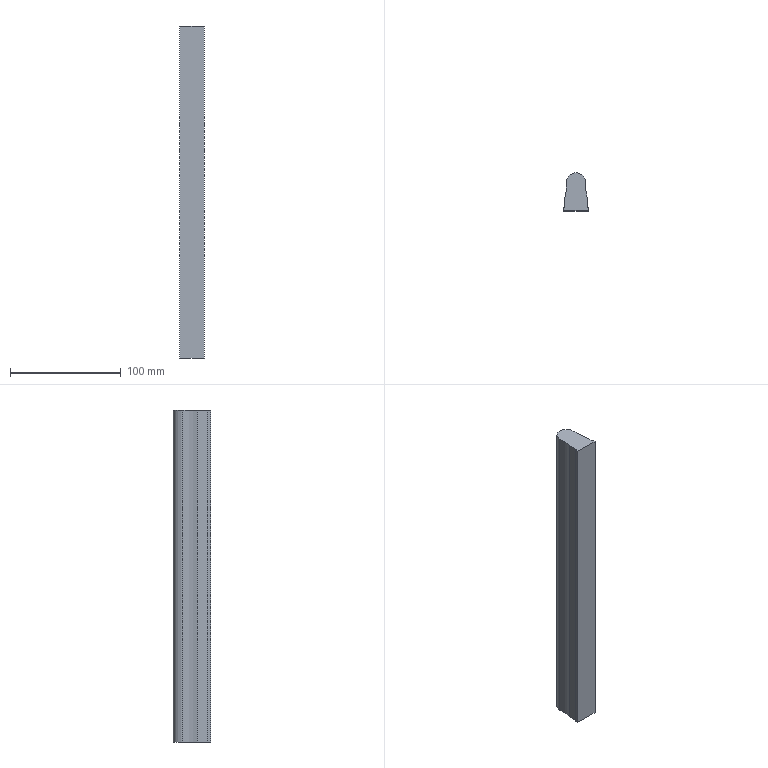Part | SolidWorks | features Extrusion 1 | 1 solid | 12 faces | box 22 x 34 x 300 mm | volume 181288 mm3 | plane 9 | spline 2 | cylinder 1 | commonest cylinder face diameters 17.6 x1
STEP:
#1=CARTESIAN_POINT('',(-8.8,25.2,0.));
#2=VERTEX_POINT('',#1);
#3=CARTESIAN_POINT('',(-10.,12.,0.));
#4=VERTEX_POINT('',#3);
#5=CARTESIAN_POINT('',(-8.8,25.2,0.));
#6=CARTESIAN_POINT('',(-8.148,18.484,0.));
#7=CARTESIAN_POINT('',(-10.,12.,0.));
#8=B_SPLINE_CURVE_WITH_KNOTS('',2,(#5,#6,#7),.UNSPECIFIED.,.F.,.F.,(3,3),(0.,1.),.UNSPECIFIED.);
#9=EDGE_CURVE('',#2,#4,#8,.T.);
#10=ORIENTED_EDGE('',*,*,#9,.T.);
#11=CARTESIAN_POINT('',(-10.,12.,300.));
#12=VERTEX_POINT('',#11);
#13=CARTESIAN_POINT('',(-10.,12.,300.));
#14=DIRECTION('',(0.,0.,-1.));
#15=VECTOR('',#14,1000.);
#16=LINE('',#13,#15);
#17=EDGE_CURVE('',#12,#4,#16,.T.);
#18=ORIENTED_EDGE('',*,*,#17,.F.);
#19=CARTESIAN_POINT('',(-8.8,25.2,300.));
#20=VERTEX_POINT('',#19);
#21=CARTESIAN_POINT('',(-8.8,25.2,300.));
#22=CARTESIAN_POINT('',(-8.148,18.484,300.));
#23=CARTESIAN_POINT('',(-10.,12.,300.));
#24=B_SPLINE_CURVE_WITH_KNOTS('',2,(#21,#22,#23),.UNSPECIFIED.,.F.,.F.,(3,3),(0.,1.),.UNSPECIFIED.);
#25=EDGE_CURVE('',#20,#12,#24,.T.);
#26=ORIENTED_EDGE('',*,*,#25,.F.);
#27=CARTESIAN_POINT('',(-8.8,25.2,300.));
#28=DIRECTION('',(0.,0.,-1.));
#29=VECTOR('',#28,1000.);
#30=LINE('',#27,#29);
#31=EDGE_CURVE('',#20,#2,#30,.T.);
#32=ORIENTED_EDGE('',*,*,#31,.T.);
#33=EDGE_LOOP('',(#10,#18,#26,#32));
#34=FACE_OUTER_BOUND('',#33,.T.);
#35=CARTESIAN_POINT('',(-8.8,25.2,300.));
#36=CARTESIAN_POINT('',(-8.8,25.2,0.));
#37=CARTESIAN_POINT('',(-8.148,18.484,300.));
#38=CARTESIAN_POINT('',(-8.148,18.484,0.));
#39=CARTESIAN_POINT('',(-10.,12.,300.));
#40=CARTESIAN_POINT('',(-10.,12.,0.));
#41=B_SPLINE_SURFACE_WITH_KNOTS('',2,1,((#35,#36),(#37,#38),(#39,#40)),.UNSPECIFIED.,.F.,.F.,.F.,(3,3),(2,2),(0.,1.),(0.,1.),.UNSPECIFIED.);
#42=ADVANCED_FACE('',(#34),#41,.F.);
#43=CARTESIAN_POINT('',(-10.,2.8,0.));
#44=VERTEX_POINT('',#43);
#45=CARTESIAN_POINT('',(-10.,12.,0.));
#46=DIRECTION('',(0.,-1.,0.));
#47=VECTOR('',#46,1000.);
#48=LINE('',#45,#47);
#49=EDGE_CURVE('',#4,#44,#48,.T.);
#50=ORIENTED_EDGE('',*,*,#49,.T.);
#51=CARTESIAN_POINT('',(-10.,2.8,300.));
#52=VERTEX_POINT('',#51);
#53=CARTESIAN_POINT('',(-10.,2.8,300.));
#54=DIRECTION('',(0.,0.,-1.));
#55=VECTOR('',#54,1000.);
#56=LINE('',#53,#55);
#57=EDGE_CURVE('',#52,#44,#56,.T.);
#58=ORIENTED_EDGE('',*,*,#57,.F.);
#59=CARTESIAN_POINT('',(-10.,12.,300.));
#60=DIRECTION('',(0.,-1.,0.));
#61=VECTOR('',#60,1000.);
#62=LINE('',#59,#61);
#63=EDGE_CURVE('',#12,#52,#62,.T.);
#64=ORIENTED_EDGE('',*,*,#63,.F.);
#65=ORIENTED_EDGE('',*,*,#17,.T.);
#66=EDGE_LOOP('',(#50,#58,#64,#65));
#67=FACE_OUTER_BOUND('',#66,.T.);
#68=CARTESIAN_POINT('',(-10.,12.,300.));
#69=DIRECTION('',(1.,0.,0.));
#70=DIRECTION('',(0.,1.,0.));
#71=AXIS2_PLACEMENT_3D('',#68,#69,#70);
#72=PLANE('',#71);
#73=ADVANCED_FACE('',(#67),#72,.F.);
#74=CARTESIAN_POINT('',(-11.,2.8,0.));
#75=VERTEX_POINT('',#74);
#76=CARTESIAN_POINT('',(-10.,2.8,0.));
#77=DIRECTION('',(-1.,0.,0.));
#78=VECTOR('',#77,1000.);
#79=LINE('',#76,#78);
#80=EDGE_CURVE('',#44,#75,#79,.T.);
#81=ORIENTED_EDGE('',*,*,#80,.T.);
#82=CARTESIAN_POINT('',(-11.,2.8,300.));
#83=VERTEX_POINT('',#82);
#84=CARTESIAN_POINT('',(-11.,2.8,300.));
#85=DIRECTION('',(0.,0.,-1.));
#86=VECTOR('',#85,1000.);
#87=LINE('',#84,#86);
#88=EDGE_CURVE('',#83,#75,#87,.T.);
#89=ORIENTED_EDGE('',*,*,#88,.F.);
#90=CARTESIAN_POINT('',(-10.,2.8,300.));
#91=DIRECTION('',(-1.,0.,0.));
#92=VECTOR('',#91,1000.);
#93=LINE('',#90,#92);
#94=EDGE_CURVE('',#52,#83,#93,.T.);
#95=ORIENTED_EDGE('',*,*,#94,.F.);
#96=ORIENTED_EDGE('',*,*,#57,.T.);
#97=EDGE_LOOP('',(#81,#89,#95,#96));
#98=FACE_OUTER_BOUND('',#97,.T.);
#99=CARTESIAN_POINT('',(-10.,2.8,300.));
#100=DIRECTION('',(0.,-1.,0.));
#101=DIRECTION('',(0.,0.,-1.));
#102=AXIS2_PLACEMENT_3D('',#99,#100,#101);
#103=PLANE('',#102);
#104=ADVANCED_FACE('',(#98),#103,.F.);
#105=CARTESIAN_POINT('',(-11.,0.,0.));
#106=VERTEX_POINT('',#105);
#107=CARTESIAN_POINT('',(-11.,2.8,0.));
#108=DIRECTION('',(0.,-1.,0.));
#109=VECTOR('',#108,1000.);
#110=LINE('',#107,#109);
#111=EDGE_CURVE('',#75,#106,#110,.T.);
#112=ORIENTED_EDGE('',*,*,#111,.T.);
#113=CARTESIAN_POINT('',(-11.,0.,300.));
#114=VERTEX_POINT('',#113);
#115=CARTESIAN_POINT('',(-11.,0.,300.));
#116=DIRECTION('',(0.,0.,-1.));
#117=VECTOR('',#116,1000.);
#118=LINE('',#115,#117);
#119=EDGE_CURVE('',#114,#106,#118,.T.);
#120=ORIENTED_EDGE('',*,*,#119,.F.);
#121=CARTESIAN_POINT('',(-11.,2.8,300.));
#122=DIRECTION('',(0.,-1.,0.));
#123=VECTOR('',#122,1000.);
#124=LINE('',#121,#123);
#125=EDGE_CURVE('',#83,#114,#124,.T.);
#126=ORIENTED_EDGE('',*,*,#125,.F.);
#127=ORIENTED_EDGE('',*,*,#88,.T.);
#128=EDGE_LOOP('',(#112,#120,#126,#127));
#129=FACE_OUTER_BOUND('',#128,.T.);
#130=CARTESIAN_POINT('',(-11.,2.8,300.));
#131=DIRECTION('',(1.,0.,0.));
#132=DIRECTION('',(0.,0.,-1.));
#133=AXIS2_PLACEMENT_3D('',#130,#131,#132);
#134=PLANE('',#133);
#135=ADVANCED_FACE('',(#129),#134,.F.);
#136=CARTESIAN_POINT('',(11.,0.,0.));
#137=VERTEX_POINT('',#136);
#138=CARTESIAN_POINT('',(11.,0.,0.));
#139=DIRECTION('',(1.,0.,0.));
#140=VECTOR('',#139,1000.);
#141=LINE('',#138,#140);
#142=EDGE_CURVE('',#106,#137,#141,.T.);
#143=ORIENTED_EDGE('',*,*,#142,.T.);
#144=CARTESIAN_POINT('',(11.,0.,300.));
#145=VERTEX_POINT('',#144);
#146=CARTESIAN_POINT('',(11.,0.,300.));
#147=DIRECTION('',(0.,0.,-1.));
#148=VECTOR('',#147,1000.);
#149=LINE('',#146,#148);
#150=EDGE_CURVE('',#145,#137,#149,.T.);
#151=ORIENTED_EDGE('',*,*,#150,.F.);
#152=CARTESIAN_POINT('',(11.,0.,300.));
#153=DIRECTION('',(1.,0.,0.));
#154=VECTOR('',#153,1000.);
#155=LINE('',#152,#154);
#156=EDGE_CURVE('',#114,#145,#155,.T.);
#157=ORIENTED_EDGE('',*,*,#156,.F.);
#158=ORIENTED_EDGE('',*,*,#119,.T.);
#159=EDGE_LOOP('',(#143,#151,#157,#158));
#160=FACE_OUTER_BOUND('',#159,.T.);
#161=CARTESIAN_POINT('',(11.,0.,300.));
#162=DIRECTION('',(0.,1.,0.));
#163=DIRECTION('',(0.,0.,1.));
#164=AXIS2_PLACEMENT_3D('',#161,#162,#163);
#165=PLANE('',#164);
#166=ADVANCED_FACE('',(#160),#165,.F.);
#167=CARTESIAN_POINT('',(11.,2.8,0.));
#168=VERTEX_POINT('',#167);
#169=CARTESIAN_POINT('',(11.,2.8,0.));
#170=DIRECTION('',(0.,1.,0.));
#171=VECTOR('',#170,1000.);
#172=LINE('',#169,#171);
#173=EDGE_CURVE('',#137,#168,#172,.T.);
#174=ORIENTED_EDGE('',*,*,#173,.T.);
#175=CARTESIAN_POINT('',(11.,2.8,300.));
#176=VERTEX_POINT('',#175);
#177=CARTESIAN_POINT('',(11.,2.8,300.));
#178=DIRECTION('',(0.,0.,-1.));
#179=VECTOR('',#178,1000.);
#180=LINE('',#177,#179);
#181=EDGE_CURVE('',#176,#168,#180,.T.);
#182=ORIENTED_EDGE('',*,*,#181,.F.);
#183=CARTESIAN_POINT('',(11.,2.8,300.));
#184=DIRECTION('',(0.,1.,0.));
#185=VECTOR('',#184,1000.);
#186=LINE('',#183,#185);
#187=EDGE_CURVE('',#145,#176,#186,.T.);
#188=ORIENTED_EDGE('',*,*,#187,.F.);
#189=ORIENTED_EDGE('',*,*,#150,.T.);
#190=EDGE_LOOP('',(#174,#182,#188,#189));
#191=FACE_OUTER_BOUND('',#190,.T.);
#192=CARTESIAN_POINT('',(11.,2.8,300.));
#193=DIRECTION('',(-1.,0.,0.));
#194=DIRECTION('',(0.,0.,1.));
#195=AXIS2_PLACEMENT_3D('',#192,#193,#194);
#196=PLANE('',#195);
#197=ADVANCED_FACE('',(#191),#196,.F.);
#198=CARTESIAN_POINT('',(10.,2.8,0.));
#199=VERTEX_POINT('',#198);
#200=CARTESIAN_POINT('',(10.,2.8,0.));
#201=DIRECTION('',(-1.,0.,0.));
#202=VECTOR('',#201,1000.);
#203=LINE('',#200,#202);
#204=EDGE_CURVE('',#168,#199,#203,.T.);
#205=ORIENTED_EDGE('',*,*,#204,.T.);
#206=CARTESIAN_POINT('',(10.,2.8,300.));
#207=VERTEX_POINT('',#206);
#208=CARTESIAN_POINT('',(10.,2.8,300.));
#209=DIRECTION('',(0.,0.,-1.));
#210=VECTOR('',#209,1000.);
#211=LINE('',#208,#210);
#212=EDGE_CURVE('',#207,#199,#211,.T.);
#213=ORIENTED_EDGE('',*,*,#212,.F.);
#214=CARTESIAN_POINT('',(10.,2.8,300.));
#215=DIRECTION('',(-1.,0.,0.));
#216=VECTOR('',#215,1000.);
#217=LINE('',#214,#216);
#218=EDGE_CURVE('',#176,#207,#217,.T.);
#219=ORIENTED_EDGE('',*,*,#218,.F.);
#220=ORIENTED_EDGE('',*,*,#181,.T.);
#221=EDGE_LOOP('',(#205,#213,#219,#220));
#222=FACE_OUTER_BOUND('',#221,.T.);
#223=CARTESIAN_POINT('',(10.,2.8,300.));
#224=DIRECTION('',(0.,-1.,0.));
#225=DIRECTION('',(0.,0.,-1.));
#226=AXIS2_PLACEMENT_3D('',#223,#224,#225);
#227=PLANE('',#226);
#228=ADVANCED_FACE('',(#222),#227,.F.);
#229=CARTESIAN_POINT('',(10.,12.,0.));
#230=VERTEX_POINT('',#229);
#231=CARTESIAN_POINT('',(10.,12.,0.));
#232=DIRECTION('',(0.,1.,0.));
#233=VECTOR('',#232,1000.);
#234=LINE('',#231,#233);
#235=EDGE_CURVE('',#199,#230,#234,.T.);
#236=ORIENTED_EDGE('',*,*,#235,.T.);
#237=CARTESIAN_POINT('',(10.,12.,300.));
#238=VERTEX_POINT('',#237);
#239=CARTESIAN_POINT('',(10.,12.,300.));
#240=DIRECTION('',(0.,0.,-1.));
#241=VECTOR('',#240,1000.);
#242=LINE('',#239,#241);
#243=EDGE_CURVE('',#238,#230,#242,.T.);
#244=ORIENTED_EDGE('',*,*,#243,.F.);
#245=CARTESIAN_POINT('',(10.,12.,300.));
#246=DIRECTION('',(0.,1.,0.));
#247=VECTOR('',#246,1000.);
#248=LINE('',#245,#247);
#249=EDGE_CURVE('',#207,#238,#248,.T.);
#250=ORIENTED_EDGE('',*,*,#249,.F.);
#251=ORIENTED_EDGE('',*,*,#212,.T.);
#252=EDGE_LOOP('',(#236,#244,#250,#251));
#253=FACE_OUTER_BOUND('',#252,.T.);
#254=CARTESIAN_POINT('',(10.,12.,300.));
#255=DIRECTION('',(-1.,0.,0.));
#256=DIRECTION('',(0.,-1.,0.));
#257=AXIS2_PLACEMENT_3D('',#254,#255,#256);
#258=PLANE('',#257);
#259=ADVANCED_FACE('',(#253),#258,.F.);
#260=CARTESIAN_POINT('',(8.8,25.2,0.));
#261=VERTEX_POINT('',#260);
#262=CARTESIAN_POINT('',(10.,12.,0.));
#263=CARTESIAN_POINT('',(8.148,18.484,0.));
#264=CARTESIAN_POINT('',(8.8,25.2,0.));
#265=B_SPLINE_CURVE_WITH_KNOTS('',2,(#262,#263,#264),.UNSPECIFIED.,.F.,.F.,(3,3),(0.,1.),.UNSPECIFIED.);
#266=EDGE_CURVE('',#230,#261,#265,.T.);
#267=ORIENTED_EDGE('',*,*,#266,.T.);
#268=CARTESIAN_POINT('',(8.8,25.2,300.));
#269=VERTEX_POINT('',#268);
#270=CARTESIAN_POINT('',(8.8,25.2,300.));
#271=DIRECTION('',(0.,0.,-1.));
#272=VECTOR('',#271,1000.);
#273=LINE('',#270,#272);
#274=EDGE_CURVE('',#269,#261,#273,.T.);
#275=ORIENTED_EDGE('',*,*,#274,.F.);
#276=CARTESIAN_POINT('',(10.,12.,300.));
#277=CARTESIAN_POINT('',(8.148,18.484,300.));
#278=CARTESIAN_POINT('',(8.8,25.2,300.));
#279=B_SPLINE_CURVE_WITH_KNOTS('',2,(#276,#277,#278),.UNSPECIFIED.,.F.,.F.,(3,3),(0.,1.),.UNSPECIFIED.);
#280=EDGE_CURVE('',#238,#269,#279,.T.);
#281=ORIENTED_EDGE('',*,*,#280,.F.);
#282=ORIENTED_EDGE('',*,*,#243,.T.);
#283=EDGE_LOOP('',(#267,#275,#281,#282));
#284=FACE_OUTER_BOUND('',#283,.T.);
#285=CARTESIAN_POINT('',(10.,12.,300.));
#286=CARTESIAN_POINT('',(10.,12.,0.));
#287=CARTESIAN_POINT('',(8.148,18.484,300.));
#288=CARTESIAN_POINT('',(8.148,18.484,0.));
#289=CARTESIAN_POINT('',(8.8,25.2,300.));
#290=CARTESIAN_POINT('',(8.8,25.2,0.));
#291=B_SPLINE_SURFACE_WITH_KNOTS('',2,1,((#285,#286),(#287,#288),(#289,#290)),.UNSPECIFIED.,.F.,.F.,.F.,(3,3),(2,2),(0.,1.),(0.,1.),.UNSPECIFIED.);
#292=ADVANCED_FACE('',(#284),#291,.F.);
#293=CARTESIAN_POINT('',(0.,25.2,0.));
#294=DIRECTION('',(0.,0.,1.));
#295=DIRECTION('',(1.,0.,0.));
#296=AXIS2_PLACEMENT_3D('',#293,#294,#295);
#297=CIRCLE('',#296,8.8);
#298=EDGE_CURVE('',#261,#2,#297,.T.);
#299=ORIENTED_EDGE('',*,*,#298,.T.);
#300=ORIENTED_EDGE('',*,*,#31,.F.);
#301=CARTESIAN_POINT('',(0.,25.2,300.));
#302=DIRECTION('',(0.,0.,1.));
#303=DIRECTION('',(1.,0.,0.));
#304=AXIS2_PLACEMENT_3D('',#301,#302,#303);
#305=CIRCLE('',#304,8.8);
#306=EDGE_CURVE('',#269,#20,#305,.T.);
#307=ORIENTED_EDGE('',*,*,#306,.F.);
#308=ORIENTED_EDGE('',*,*,#274,.T.);
#309=EDGE_LOOP('',(#299,#300,#307,#308));
#310=FACE_OUTER_BOUND('',#309,.T.);
#311=CARTESIAN_POINT('',(0.,25.2,300.));
#312=DIRECTION('',(0.,0.,-1.));
#313=DIRECTION('',(-1.,0.,0.));
#314=AXIS2_PLACEMENT_3D('',#311,#312,#313);
#315=CYLINDRICAL_SURFACE('',#314,8.8);
#316=ADVANCED_FACE('',(#310),#315,.T.);
#317=ORIENTED_EDGE('',*,*,#25,.T.);
#318=ORIENTED_EDGE('',*,*,#63,.T.);
#319=ORIENTED_EDGE('',*,*,#94,.T.);
#320=ORIENTED_EDGE('',*,*,#125,.T.);
#321=ORIENTED_EDGE('',*,*,#156,.T.);
#322=ORIENTED_EDGE('',*,*,#187,.T.);
#323=ORIENTED_EDGE('',*,*,#218,.T.);
#324=ORIENTED_EDGE('',*,*,#249,.T.);
#325=ORIENTED_EDGE('',*,*,#280,.T.);
#326=ORIENTED_EDGE('',*,*,#306,.T.);
#327=EDGE_LOOP('',(#317,#318,#319,#320,#321,#322,#323,#324,#325,#326));
#328=FACE_OUTER_BOUND('',#327,.T.);
#329=CARTESIAN_POINT('',(-8.774,18.542,300.));
#330=DIRECTION('',(0.,0.,1.));
#331=DIRECTION('',(1.,0.,0.));
#332=AXIS2_PLACEMENT_3D('',#329,#330,#331);
#333=PLANE('',#332);
#334=ADVANCED_FACE('',(#328),#333,.T.);
#335=ORIENTED_EDGE('',*,*,#9,.F.);
#336=ORIENTED_EDGE('',*,*,#298,.F.);
#337=ORIENTED_EDGE('',*,*,#266,.F.);
#338=ORIENTED_EDGE('',*,*,#235,.F.);
#339=ORIENTED_EDGE('',*,*,#204,.F.);
#340=ORIENTED_EDGE('',*,*,#173,.F.);
#341=ORIENTED_EDGE('',*,*,#142,.F.);
#342=ORIENTED_EDGE('',*,*,#111,.F.);
#343=ORIENTED_EDGE('',*,*,#80,.F.);
#344=ORIENTED_EDGE('',*,*,#49,.F.);
#345=EDGE_LOOP('',(#335,#336,#337,#338,#339,#340,#341,#342,#343,#344));
#346=FACE_OUTER_BOUND('',#345,.T.);
#347=CARTESIAN_POINT('',(-8.774,18.542,0.));
#348=DIRECTION('',(0.,0.,1.));
#349=DIRECTION('',(1.,0.,0.));
#350=AXIS2_PLACEMENT_3D('',#347,#348,#349);
#351=PLANE('',#350);
#352=ADVANCED_FACE('',(#346),#351,.F.);
#353=CLOSED_SHELL('',(#42,#73,#104,#135,#166,#197,#228,#259,#292,#316,#334,#352));
#354=MANIFOLD_SOLID_BREP('',#353);
#355=CARTESIAN_POINT('',(0.,0.,0.));
#356=DIRECTION('',(0.,0.,1.));
#357=DIRECTION('',(1.,0.,0.));
#358=AXIS2_PLACEMENT_3D('',#355,#356,#357);
#359=(LENGTH_UNIT()NAMED_UNIT(*)SI_UNIT(.MILLI.,.METRE.));
#360=UNCERTAINTY_MEASURE_WITH_UNIT(LENGTH_MEASURE(0.00001),#359,'','');
#361=(NAMED_UNIT(*)PLANE_ANGLE_UNIT()SI_UNIT($,.RADIAN.));
#362=(NAMED_UNIT(*)SI_UNIT($,.STERADIAN.)SOLID_ANGLE_UNIT());
#363=(GEOMETRIC_REPRESENTATION_CONTEXT(3)GLOBAL_UNCERTAINTY_ASSIGNED_CONTEXT((#360))GLOBAL_UNIT_ASSIGNED_CONTEXT((#359,#361,#362))REPRESENTATION_CONTEXT('',''));
#364=ADVANCED_BREP_SHAPE_REPRESENTATION('',(#354,#358),#363);